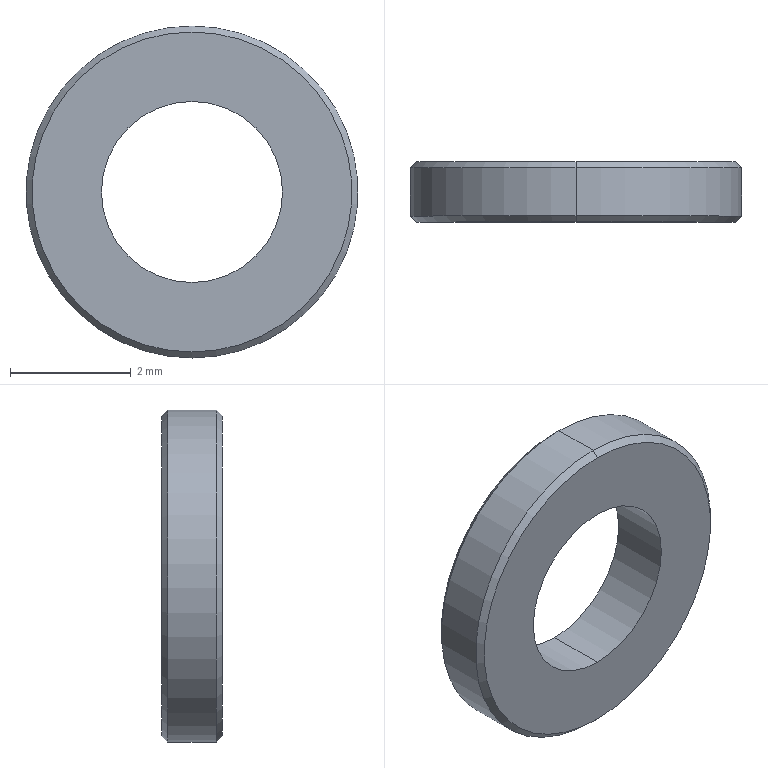Part | SolidWorks | features Chamfer 1, Extrusion 1 | 1 solid | 10 faces | box 5.5 x 1 x 5.5 mm | volume 16.519 mm3 | cone 4 | cylinder 4 | plane 2 | commonest cylinder face diameters 3 x2 5.5 x2
STEP:
#1=CARTESIAN_POINT('',(0.,1.,2.65));
#2=VERTEX_POINT('',#1);
#3=CARTESIAN_POINT('',(0.,1.,-2.65));
#4=VERTEX_POINT('',#3);
#5=CARTESIAN_POINT('',(0.,1.,0.));
#6=DIRECTION('',(0.,1.,0.));
#7=DIRECTION('',(0.,0.,1.));
#8=AXIS2_PLACEMENT_3D('',#5,#6,#7);
#9=CIRCLE('',#8,2.65);
#10=EDGE_CURVE('',#2,#4,#9,.T.);
#11=ORIENTED_EDGE('',*,*,#10,.F.);
#12=CARTESIAN_POINT('',(0.,0.9,2.75));
#13=VERTEX_POINT('',#12);
#14=CARTESIAN_POINT('',(0.,1.,2.65));
#15=DIRECTION('',(0.,-0.7071,0.7071));
#16=VECTOR('',#15,1000.);
#17=LINE('',#14,#16);
#18=EDGE_CURVE('',#2,#13,#17,.T.);
#19=ORIENTED_EDGE('',*,*,#18,.T.);
#20=CARTESIAN_POINT('',(0.,0.9,-2.75));
#21=VERTEX_POINT('',#20);
#22=CARTESIAN_POINT('',(0.,0.9,0.));
#23=DIRECTION('',(0.,-1.,0.));
#24=DIRECTION('',(0.,0.,1.));
#25=AXIS2_PLACEMENT_3D('',#22,#23,#24);
#26=CIRCLE('',#25,2.75);
#27=EDGE_CURVE('',#21,#13,#26,.T.);
#28=ORIENTED_EDGE('',*,*,#27,.F.);
#29=CARTESIAN_POINT('',(0.,1.,-2.65));
#30=DIRECTION('',(0.,-0.7071,-0.7071));
#31=VECTOR('',#30,1000.);
#32=LINE('',#29,#31);
#33=EDGE_CURVE('',#4,#21,#32,.T.);
#34=ORIENTED_EDGE('',*,*,#33,.F.);
#35=EDGE_LOOP('',(#11,#19,#28,#34));
#36=FACE_OUTER_BOUND('',#35,.T.);
#37=CARTESIAN_POINT('',(0.,1.,0.));
#38=DIRECTION('',(0.,-1.,0.));
#39=DIRECTION('',(0.,0.,-1.));
#40=AXIS2_PLACEMENT_3D('',#37,#38,#39);
#41=CONICAL_SURFACE('',#40,2.65,0.7854);
#42=ADVANCED_FACE('',(#36),#41,.T.);
#43=CARTESIAN_POINT('',(0.,0.,-2.65));
#44=VERTEX_POINT('',#43);
#45=CARTESIAN_POINT('',(0.,0.,2.65));
#46=VERTEX_POINT('',#45);
#47=CARTESIAN_POINT('',(0.,0.,0.));
#48=DIRECTION('',(0.,-1.,0.));
#49=DIRECTION('',(0.,0.,1.));
#50=AXIS2_PLACEMENT_3D('',#47,#48,#49);
#51=CIRCLE('',#50,2.65);
#52=EDGE_CURVE('',#44,#46,#51,.T.);
#53=ORIENTED_EDGE('',*,*,#52,.F.);
#54=CARTESIAN_POINT('',(0.,0.1,-2.75));
#55=VERTEX_POINT('',#54);
#56=CARTESIAN_POINT('',(0.,0.1,-2.75));
#57=DIRECTION('',(0.,0.7071,-0.7071));
#58=VECTOR('',#57,1000.);
#59=LINE('',#56,#58);
#60=EDGE_CURVE('',#44,#55,#59,.T.);
#61=ORIENTED_EDGE('',*,*,#60,.T.);
#62=CARTESIAN_POINT('',(0.,0.1,2.75));
#63=VERTEX_POINT('',#62);
#64=CARTESIAN_POINT('',(0.,0.1,0.));
#65=DIRECTION('',(0.,1.,0.));
#66=DIRECTION('',(0.,0.,1.));
#67=AXIS2_PLACEMENT_3D('',#64,#65,#66);
#68=CIRCLE('',#67,2.75);
#69=EDGE_CURVE('',#63,#55,#68,.T.);
#70=ORIENTED_EDGE('',*,*,#69,.F.);
#71=CARTESIAN_POINT('',(0.,0.1,2.75));
#72=DIRECTION('',(0.,0.7071,0.7071));
#73=VECTOR('',#72,1000.);
#74=LINE('',#71,#73);
#75=EDGE_CURVE('',#46,#63,#74,.T.);
#76=ORIENTED_EDGE('',*,*,#75,.F.);
#77=EDGE_LOOP('',(#53,#61,#70,#76));
#78=FACE_OUTER_BOUND('',#77,.T.);
#79=CARTESIAN_POINT('',(0.,0.1,0.));
#80=DIRECTION('',(0.,1.,0.));
#81=DIRECTION('',(0.,0.,1.));
#82=AXIS2_PLACEMENT_3D('',#79,#80,#81);
#83=CONICAL_SURFACE('',#82,2.75,0.7854);
#84=ADVANCED_FACE('',(#78),#83,.T.);
#85=CARTESIAN_POINT('',(0.,1.,-1.5));
#86=VERTEX_POINT('',#85);
#87=CARTESIAN_POINT('',(0.,1.,1.5));
#88=VERTEX_POINT('',#87);
#89=CARTESIAN_POINT('',(0.,1.,0.));
#90=DIRECTION('',(0.,1.,0.));
#91=DIRECTION('',(0.,0.,1.));
#92=AXIS2_PLACEMENT_3D('',#89,#90,#91);
#93=CIRCLE('',#92,1.5);
#94=EDGE_CURVE('',#86,#88,#93,.T.);
#95=ORIENTED_EDGE('',*,*,#94,.T.);
#96=CARTESIAN_POINT('',(0.,0.,1.5));
#97=VERTEX_POINT('',#96);
#98=CARTESIAN_POINT('',(0.,1.,1.5));
#99=DIRECTION('',(0.,-1.,0.));
#100=VECTOR('',#99,1000.);
#101=LINE('',#98,#100);
#102=EDGE_CURVE('',#88,#97,#101,.T.);
#103=ORIENTED_EDGE('',*,*,#102,.T.);
#104=CARTESIAN_POINT('',(0.,0.,-1.5));
#105=VERTEX_POINT('',#104);
#106=CARTESIAN_POINT('',(0.,0.,0.));
#107=DIRECTION('',(0.,1.,0.));
#108=DIRECTION('',(0.,0.,1.));
#109=AXIS2_PLACEMENT_3D('',#106,#107,#108);
#110=CIRCLE('',#109,1.5);
#111=EDGE_CURVE('',#105,#97,#110,.T.);
#112=ORIENTED_EDGE('',*,*,#111,.F.);
#113=CARTESIAN_POINT('',(0.,1.,-1.5));
#114=DIRECTION('',(0.,-1.,0.));
#115=VECTOR('',#114,1000.);
#116=LINE('',#113,#115);
#117=EDGE_CURVE('',#86,#105,#116,.T.);
#118=ORIENTED_EDGE('',*,*,#117,.F.);
#119=EDGE_LOOP('',(#95,#103,#112,#118));
#120=FACE_OUTER_BOUND('',#119,.T.);
#121=CARTESIAN_POINT('',(0.,1.,0.));
#122=DIRECTION('',(0.,-1.,0.));
#123=DIRECTION('',(0.,0.,-1.));
#124=AXIS2_PLACEMENT_3D('',#121,#122,#123);
#125=CYLINDRICAL_SURFACE('',#124,1.5);
#126=ADVANCED_FACE('',(#120),#125,.F.);
#127=ORIENTED_EDGE('',*,*,#27,.T.);
#128=CARTESIAN_POINT('',(0.,1.,2.75));
#129=DIRECTION('',(0.,-1.,0.));
#130=VECTOR('',#129,1000.);
#131=LINE('',#128,#130);
#132=EDGE_CURVE('',#13,#63,#131,.T.);
#133=ORIENTED_EDGE('',*,*,#132,.T.);
#134=ORIENTED_EDGE('',*,*,#69,.T.);
#135=CARTESIAN_POINT('',(0.,1.,-2.75));
#136=DIRECTION('',(0.,-1.,0.));
#137=VECTOR('',#136,1000.);
#138=LINE('',#135,#137);
#139=EDGE_CURVE('',#21,#55,#138,.T.);
#140=ORIENTED_EDGE('',*,*,#139,.F.);
#141=EDGE_LOOP('',(#127,#133,#134,#140));
#142=FACE_OUTER_BOUND('',#141,.T.);
#143=CARTESIAN_POINT('',(0.,1.,0.));
#144=DIRECTION('',(0.,-1.,0.));
#145=DIRECTION('',(0.,0.,-1.));
#146=AXIS2_PLACEMENT_3D('',#143,#144,#145);
#147=CYLINDRICAL_SURFACE('',#146,2.75);
#148=ADVANCED_FACE('',(#142),#147,.T.);
#149=CARTESIAN_POINT('',(0.,1.,0.));
#150=DIRECTION('',(0.,1.,0.));
#151=DIRECTION('',(0.,0.,1.));
#152=AXIS2_PLACEMENT_3D('',#149,#150,#151);
#153=CIRCLE('',#152,2.65);
#154=EDGE_CURVE('',#4,#2,#153,.T.);
#155=ORIENTED_EDGE('',*,*,#154,.T.);
#156=ORIENTED_EDGE('',*,*,#10,.T.);
#157=EDGE_LOOP('',(#155,#156));
#158=FACE_OUTER_BOUND('',#157,.T.);
#159=ORIENTED_EDGE('',*,*,#94,.F.);
#160=CARTESIAN_POINT('',(0.,1.,0.));
#161=DIRECTION('',(0.,1.,0.));
#162=DIRECTION('',(0.,0.,1.));
#163=AXIS2_PLACEMENT_3D('',#160,#161,#162);
#164=CIRCLE('',#163,1.5);
#165=EDGE_CURVE('',#88,#86,#164,.T.);
#166=ORIENTED_EDGE('',*,*,#165,.F.);
#167=EDGE_LOOP('',(#159,#166));
#168=FACE_BOUND('',#167,.T.);
#169=CARTESIAN_POINT('',(0.,1.,0.));
#170=DIRECTION('',(0.,1.,0.));
#171=DIRECTION('',(0.,0.,1.));
#172=AXIS2_PLACEMENT_3D('',#169,#170,#171);
#173=PLANE('',#172);
#174=ADVANCED_FACE('',(#158,#168),#173,.T.);
#175=CARTESIAN_POINT('',(0.,0.,0.));
#176=DIRECTION('',(0.,-1.,0.));
#177=DIRECTION('',(0.,0.,1.));
#178=AXIS2_PLACEMENT_3D('',#175,#176,#177);
#179=CIRCLE('',#178,2.65);
#180=EDGE_CURVE('',#46,#44,#179,.T.);
#181=ORIENTED_EDGE('',*,*,#180,.T.);
#182=ORIENTED_EDGE('',*,*,#52,.T.);
#183=EDGE_LOOP('',(#181,#182));
#184=FACE_OUTER_BOUND('',#183,.T.);
#185=ORIENTED_EDGE('',*,*,#111,.T.);
#186=CARTESIAN_POINT('',(0.,0.,0.));
#187=DIRECTION('',(0.,1.,0.));
#188=DIRECTION('',(0.,0.,1.));
#189=AXIS2_PLACEMENT_3D('',#186,#187,#188);
#190=CIRCLE('',#189,1.5);
#191=EDGE_CURVE('',#97,#105,#190,.T.);
#192=ORIENTED_EDGE('',*,*,#191,.T.);
#193=EDGE_LOOP('',(#185,#192));
#194=FACE_BOUND('',#193,.T.);
#195=CARTESIAN_POINT('',(0.,0.,0.));
#196=DIRECTION('',(0.,1.,0.));
#197=DIRECTION('',(0.,0.,1.));
#198=AXIS2_PLACEMENT_3D('',#195,#196,#197);
#199=PLANE('',#198);
#200=ADVANCED_FACE('',(#184,#194),#199,.F.);
#201=ORIENTED_EDGE('',*,*,#132,.F.);
#202=CARTESIAN_POINT('',(0.,0.9,0.));
#203=DIRECTION('',(0.,-1.,0.));
#204=DIRECTION('',(0.,0.,1.));
#205=AXIS2_PLACEMENT_3D('',#202,#203,#204);
#206=CIRCLE('',#205,2.75);
#207=EDGE_CURVE('',#13,#21,#206,.T.);
#208=ORIENTED_EDGE('',*,*,#207,.T.);
#209=ORIENTED_EDGE('',*,*,#139,.T.);
#210=CARTESIAN_POINT('',(0.,0.1,0.));
#211=DIRECTION('',(0.,1.,0.));
#212=DIRECTION('',(0.,0.,1.));
#213=AXIS2_PLACEMENT_3D('',#210,#211,#212);
#214=CIRCLE('',#213,2.75);
#215=EDGE_CURVE('',#55,#63,#214,.T.);
#216=ORIENTED_EDGE('',*,*,#215,.T.);
#217=EDGE_LOOP('',(#201,#208,#209,#216));
#218=FACE_OUTER_BOUND('',#217,.T.);
#219=CARTESIAN_POINT('',(0.,1.,0.));
#220=DIRECTION('',(0.,-1.,0.));
#221=DIRECTION('',(0.,0.,-1.));
#222=AXIS2_PLACEMENT_3D('',#219,#220,#221);
#223=CYLINDRICAL_SURFACE('',#222,2.75);
#224=ADVANCED_FACE('',(#218),#223,.T.);
#225=ORIENTED_EDGE('',*,*,#102,.F.);
#226=ORIENTED_EDGE('',*,*,#165,.T.);
#227=ORIENTED_EDGE('',*,*,#117,.T.);
#228=ORIENTED_EDGE('',*,*,#191,.F.);
#229=EDGE_LOOP('',(#225,#226,#227,#228));
#230=FACE_OUTER_BOUND('',#229,.T.);
#231=CARTESIAN_POINT('',(0.,1.,0.));
#232=DIRECTION('',(0.,-1.,0.));
#233=DIRECTION('',(0.,0.,-1.));
#234=AXIS2_PLACEMENT_3D('',#231,#232,#233);
#235=CYLINDRICAL_SURFACE('',#234,1.5);
#236=ADVANCED_FACE('',(#230),#235,.F.);
#237=ORIENTED_EDGE('',*,*,#60,.F.);
#238=ORIENTED_EDGE('',*,*,#180,.F.);
#239=ORIENTED_EDGE('',*,*,#75,.T.);
#240=ORIENTED_EDGE('',*,*,#215,.F.);
#241=EDGE_LOOP('',(#237,#238,#239,#240));
#242=FACE_OUTER_BOUND('',#241,.T.);
#243=CARTESIAN_POINT('',(0.,0.1,0.));
#244=DIRECTION('',(0.,1.,0.));
#245=DIRECTION('',(0.,0.,1.));
#246=AXIS2_PLACEMENT_3D('',#243,#244,#245);
#247=CONICAL_SURFACE('',#246,2.75,0.7854);
#248=ADVANCED_FACE('',(#242),#247,.T.);
#249=ORIENTED_EDGE('',*,*,#18,.F.);
#250=ORIENTED_EDGE('',*,*,#154,.F.);
#251=ORIENTED_EDGE('',*,*,#33,.T.);
#252=ORIENTED_EDGE('',*,*,#207,.F.);
#253=EDGE_LOOP('',(#249,#250,#251,#252));
#254=FACE_OUTER_BOUND('',#253,.T.);
#255=CARTESIAN_POINT('',(0.,1.,0.));
#256=DIRECTION('',(0.,-1.,0.));
#257=DIRECTION('',(0.,0.,-1.));
#258=AXIS2_PLACEMENT_3D('',#255,#256,#257);
#259=CONICAL_SURFACE('',#258,2.65,0.7854);
#260=ADVANCED_FACE('',(#254),#259,.T.);
#261=CLOSED_SHELL('',(#42,#84,#126,#148,#174,#200,#224,#236,#248,#260));
#262=MANIFOLD_SOLID_BREP('',#261);
#263=CARTESIAN_POINT('',(0.,0.,0.));
#264=DIRECTION('',(0.,0.,1.));
#265=DIRECTION('',(1.,0.,0.));
#266=AXIS2_PLACEMENT_3D('',#263,#264,#265);
#267=(LENGTH_UNIT()NAMED_UNIT(*)SI_UNIT(.MILLI.,.METRE.));
#268=UNCERTAINTY_MEASURE_WITH_UNIT(LENGTH_MEASURE(0.00001),#267,'','');
#269=(NAMED_UNIT(*)PLANE_ANGLE_UNIT()SI_UNIT($,.RADIAN.));
#270=(NAMED_UNIT(*)SI_UNIT($,.STERADIAN.)SOLID_ANGLE_UNIT());
#271=(GEOMETRIC_REPRESENTATION_CONTEXT(3)GLOBAL_UNCERTAINTY_ASSIGNED_CONTEXT((#268))GLOBAL_UNIT_ASSIGNED_CONTEXT((#267,#269,#270))REPRESENTATION_CONTEXT('',''));
#272=ADVANCED_BREP_SHAPE_REPRESENTATION('',(#262,#266),#271);